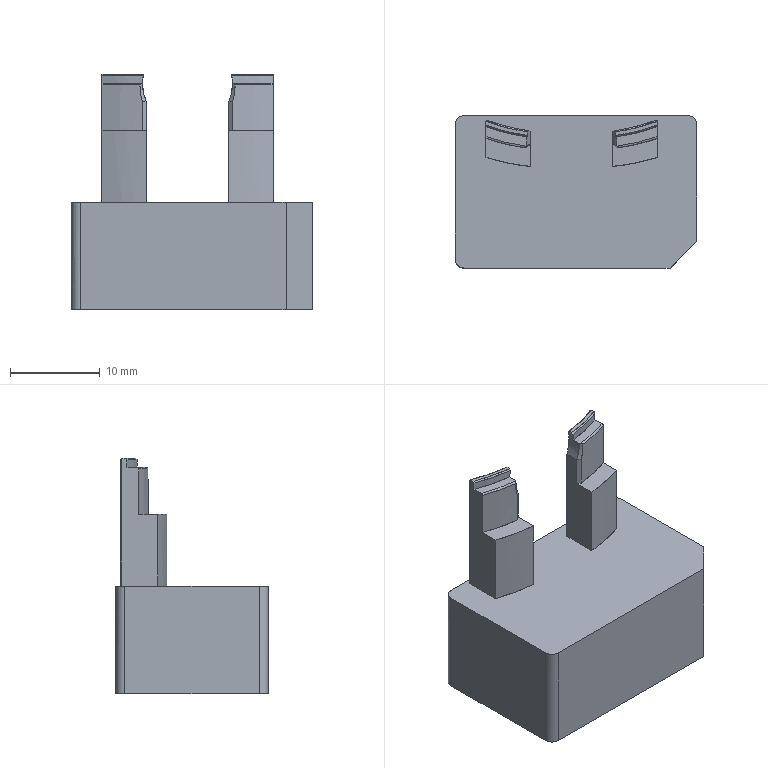NC program | PowerMill | posted by the shop | part box 27 x 17 x 26.255 mm
Lines 6760 to 8398 of 169183:
( TOOL ID   D3C_1_1 )
( TOOL DIA. 3. TIP RAD 0 LENGTH 69.44 )
( Z = -14.38 )
T15 M6
T3
G91 G28 Z0
G0 G90 G54
M08
S18000 M3
X0 Y0 M8
G43 Z9.805 H15
X-7.381 Y9.693
Z.857
G1 Z-.343 F3000
X-7.393 Y9.677 F5000
G3 X-7.362 Y9.434 I.137 J-.106
G1 X-6.118 Y8.476
X-5.066 Y8.271
X-4.643 Y8.086
X-4.32 Y7.809
X-4.221 Y7.684
X-4.059 Y7.387
X-3.949 Y6.965
X-3.924 Y6.543
X-3.932 Y6.121
X-4.017 Y5.699
X-4.221 Y5.28
X-4.675 Y4.855
X-5.066 Y4.689
X-5.488 Y4.639
X-6.754 Y4.824
X-8.021 Y5.089
X-9.287 Y5.43
X-10.553 Y5.853
X-10.975 Y6.085
X-11.398 Y6.604
X-11.518 Y6.965
X-11.552 Y7.387
Y7.809
X-11.511 Y8.232
X-11.347 Y8.654
X-11.004 Y9.076
X-10.553 Y9.353
X-10.131 Y9.46
X-9.709 Y9.452
X-8.556 Y9.076
X-7.176 Y8.683
X-7.17 Y8.682
X-6.118 Y8.476
X-7.382 Y9.701 Z-.481
X-7.394 Y9.686
G3 X-7.363 Y9.443 I.137 J-.106
G1 X-6.117 Y8.478
X-5.066 Y8.271
X-4.643 Y8.086
X-4.32 Y7.809
X-4.221 Y7.684
X-4.059 Y7.387
X-3.949 Y6.965
X-3.924 Y6.543
X-3.932 Y6.121
X-4.017 Y5.699
X-4.221 Y5.277
X-4.424 Y5.042
X-4.671 Y4.855
X-5.066 Y4.686
X-5.488 Y4.636
X-6.332 Y4.749
X-7.024 Y4.879
X-7.712 Y5.025
X-8.021 Y5.086
X-9.287 Y5.427
X-10.553 Y5.85
X-10.975 Y6.082
X-11.398 Y6.601
X-11.521 Y6.965
X-11.552 Y7.387
Y7.809
X-11.511 Y8.232
X-11.347 Y8.654
X-11.004 Y9.076
X-10.553 Y9.353
X-10.131 Y9.46
X-9.709 Y9.452
X-9.287 Y9.334
X-8.545 Y9.076
X-7.176 Y8.688
X-6.117 Y8.478
X-7.37 Y9.699 Z-.619
X-7.382 Y9.684
G3 X-7.351 Y9.44 I.137 J-.106
G1 X-6.117 Y8.481
X-5.066 Y8.271
X-4.643 Y8.086
X-4.32 Y7.809
X-4.221 Y7.684
X-4.059 Y7.387
X-3.949 Y6.965
X-3.924 Y6.543
X-3.932 Y6.121
X-4.017 Y5.699
X-4.221 Y5.277
X-4.424 Y5.042
X-4.671 Y4.855
X-5.066 Y4.686
X-5.488 Y4.636
X-6.332 Y4.749
X-6.585 Y4.799
X-6.589 Y4.8
X-6.754 Y4.824
X-7.704 Y5.023
X-8.021 Y5.086
X-9.287 Y5.427
X-10.553 Y5.85
X-10.975 Y6.082
X-11.36 Y6.543
X-11.374 Y6.575
X-11.398 Y6.601
X-11.504 Y6.917
X-11.524 Y6.969
X-11.525 Y7.025
X-11.552 Y7.387
Y7.808
Y7.809
X-11.511 Y8.232
X-11.347 Y8.654
X-11.004 Y9.076
X-10.553 Y9.353
X-10.131 Y9.46
X-9.709 Y9.452
X-9.287 Y9.334
X-8.544 Y9.076
X-7.176 Y8.692
X-6.117 Y8.481
X-7.364 Y9.698 Z-.756
X-7.376 Y9.683
G3 X-7.346 Y9.44 I.137 J-.106
G1 X-6.117 Y8.482
X-5.066 Y8.271
X-4.643 Y8.086
X-4.32 Y7.809
X-4.221 Y7.684
X-4.059 Y7.387
X-3.949 Y6.965
X-3.924 Y6.543
X-3.932 Y6.121
X-4.017 Y5.699
X-4.221 Y5.277
X-4.424 Y5.042
X-4.671 Y4.855
X-5.066 Y4.686
X-5.488 Y4.636
X-6.332 Y4.749
X-6.586 Y4.8
X-6.59
X-6.754 Y4.824
X-7.697 Y5.022
X-8.021 Y5.086
X-9.287 Y5.427
X-10.553 Y5.85
X-10.975 Y6.082
X-11.362 Y6.543
X-11.375 Y6.575
X-11.398 Y6.602
X-11.458 Y6.785
X-11.525 Y6.965
X-11.534 Y7.177
X-11.552 Y7.387
Y7.806
Y7.809
X-11.511 Y8.232
X-11.347 Y8.654
X-11.004 Y9.076
X-10.553 Y9.353
X-10.131 Y9.46
X-9.709 Y9.452
X-9.287 Y9.334
X-8.543 Y9.076
X-7.176 Y8.695
X-6.117 Y8.482
X-7.364 Y9.698 Z-.894
X-7.375 Y9.683
G3 X-7.345 Y9.44 I.137 J-.107
G1 X-6.117 Y8.482
X-5.066 Y8.271
X-4.643 Y8.086
X-4.32 Y7.809
X-4.221 Y7.684
X-4.059 Y7.387
X-3.949 Y6.965
X-3.924 Y6.543
X-3.932 Y6.121
X-4.017 Y5.699
X-4.221 Y5.277
X-4.424 Y5.042
X-4.671 Y4.855
X-5.066 Y4.686
X-5.488 Y4.636
X-6.332 Y4.749
X-7.177 Y4.912
X-8.021 Y5.086
X-9.287 Y5.427
X-10.553 Y5.85
X-10.975 Y6.082
X-11.364 Y6.543
X-11.376 Y6.575
X-11.397 Y6.602
X-11.459 Y6.785
X-11.528 Y6.965
X-11.535 Y7.177
X-11.552 Y7.387
Y7.804
Y7.809
X-11.511 Y8.232
X-11.347 Y8.654
X-11.004 Y9.076
X-10.553 Y9.353
X-10.131 Y9.46
X-9.709 Y9.452
X-9.287 Y9.334
X-8.542 Y9.076
X-7.176 Y8.695
X-7.171 Y8.694
X-6.117 Y8.482
X-7.363 Y9.699 Z-1.032
X-7.375 Y9.684
G3 X-7.345 Y9.441 I.137 J-.107
G1 X-6.117 Y8.482
X-5.066 Y8.271
X-4.643 Y8.086
X-4.32 Y7.809
X-4.221 Y7.684
X-4.059 Y7.387
X-3.949 Y6.965
X-3.924 Y6.543
X-3.932 Y6.121
X-4.017 Y5.699
X-4.221 Y5.277
X-4.424 Y5.042
X-4.671 Y4.855
X-5.066 Y4.686
X-5.488 Y4.636
X-6.332 Y4.749
X-7.009 Y4.877
X-7.683 Y5.019
X-8.021 Y5.086
X-9.287 Y5.427
X-10.553 Y5.85
X-10.975 Y6.082
X-11.366 Y6.543
X-11.418 Y6.656
X-11.456 Y6.773
X-11.53 Y6.965
X-11.536 Y7.177
X-11.552 Y7.387
Y7.802
Y7.809
X-11.511 Y8.232
X-11.347 Y8.654
X-11.004 Y9.076
X-10.553 Y9.353
X-10.131 Y9.46
X-9.709 Y9.452
X-9.287 Y9.334
X-8.515 Y9.068
X-7.319 Y8.735
X-7.176 Y8.696
X-6.117 Y8.482
X-7.367 Y9.703 Z-1.17
X-7.378 Y9.687
G3 X-7.348 Y9.444 I.137 J-.107
G1 X-6.116 Y8.483
X-5.066 Y8.271
X-4.643 Y8.086
X-4.32 Y7.809
X-4.221 Y7.684
X-4.059 Y7.387
X-3.949 Y6.965
X-3.924 Y6.543
X-3.932 Y6.121
X-4.017 Y5.699
X-4.221 Y5.277
X-4.424 Y5.042
X-4.671 Y4.855
X-5.066 Y4.686
X-5.488 Y4.636
X-6.332 Y4.749
X-7.005 Y4.876
X-7.676 Y5.017
X-8.021 Y5.086
X-9.287 Y5.427
X-10.553 Y5.85
X-10.557 Y5.852
X-10.975 Y6.082
X-10.999 Y6.106
X-11.03 Y6.121
X-11.369 Y6.543
X-11.408 Y6.633
X-11.439 Y6.726
X-11.532 Y6.965
X-11.548 Y7.387
X-11.552 Y7.809
X-11.511 Y8.232
X-11.347 Y8.654
X-11.004 Y9.076
X-10.553 Y9.353
X-10.131 Y9.46
X-9.709 Y9.452
X-9.287 Y9.334
X-8.491 Y9.062
X-7.534 Y8.795
X-7.176 Y8.696
X-6.116 Y8.483
X-7.366 Y9.702 Z-1.32
X-7.378 Y9.687
G3 X-7.348 Y9.444 I.137 J-.107
G1 X-6.116 Y8.483
X-5.066 Y8.271
X-4.643 Y8.086
X-4.32 Y7.809
X-4.221 Y7.684
X-4.059 Y7.387
X-3.949 Y6.965
X-3.923 Y6.543
X-3.932 Y6.121
X-4.017 Y5.699
Y5.688
X-4.057 Y4.855
X-4.221 Y4.432
X-4.643 Y3.953
X-5.153 Y3.588
X-5.488 Y3.475
X-5.91 Y3.447
X-7.598 Y3.74
X-9.287 Y4.154
X-10.553 Y4.552
X-10.975 Y4.784
X-11.059 Y4.855
X-11.384 Y5.277
X-11.527 Y5.699
X-11.552 Y6.121
Y7.809
X-11.511 Y8.232
X-11.347 Y8.654
X-11.004 Y9.076
X-10.553 Y9.353
X-10.131 Y9.46
X-9.709 Y9.452
X-9.287 Y9.334
X-8.532 Y9.076
X-7.176 Y8.697
X-7.171 Y8.696
X-6.116 Y8.483
X-7.366 Y9.702 Z-1.47
X-7.378 Y9.687
G3 X-7.348 Y9.444 I.137 J-.107
G1 X-6.116 Y8.483
X-5.066 Y8.271
X-4.643 Y8.086
X-4.32 Y7.809
X-4.221 Y7.684
X-4.059 Y7.387
X-3.949 Y6.965
X-3.923 Y6.543
X-3.932 Y6.121
X-4.008 Y5.699
X-4.014 Y5.277
X-4.052 Y4.855
X-4.221 Y4.43
X-4.576 Y4.01
X-4.726 Y3.891
X-4.883 Y3.782
X-5.142 Y3.588
X-5.488 Y3.465
X-5.91 Y3.437
X-6.922 Y3.588
X-8.021 Y3.811
X-9.287 Y4.132
X-10.553 Y4.53
X-10.975 Y4.762
X-11.083 Y4.855
X-11.395 Y5.277
X-11.532 Y5.699
X-11.552 Y6.121
Y7.809
X-11.511 Y8.232
X-11.347 Y8.654
X-11.004 Y9.076
X-10.553 Y9.353
X-10.131 Y9.46
X-9.709 Y9.452
X-9.287 Y9.334
X-8.532 Y9.076
X-7.176 Y8.697
X-6.116 Y8.483
X-7.366 Y9.702 Z-1.62
X-7.378 Y9.687
G3 X-7.348 Y9.444 I.137 J-.107
G1 X-6.116 Y8.483
X-5.066 Y8.271
X-4.643 Y8.086
X-4.32 Y7.809
X-4.221 Y7.684
X-4.059 Y7.387
X-3.949 Y6.965
X-3.923 Y6.543
X-3.932 Y6.121
X-3.997 Y5.699
X-4.004 Y5.277
X-4.045 Y4.855
X-4.214 Y4.432
X-4.576 Y4.01
X-4.693 Y3.917
X-4.815 Y3.83
X-5.136 Y3.588
X-5.488 Y3.462
X-5.91 Y3.436
X-6.922 Y3.588
X-8.021 Y3.811
X-9.287 Y4.132
X-10.553 Y4.53
X-10.975 Y4.762
X-11.083 Y4.855
X-11.395 Y5.277
X-11.532 Y5.699
X-11.552 Y6.121
Y7.809
X-11.511 Y8.232
X-11.347 Y8.654
X-11.004 Y9.076
X-10.553 Y9.353
X-10.131 Y9.46
X-9.709 Y9.452
X-9.287 Y9.334
X-8.532 Y9.076
X-7.176 Y8.697
X-6.116 Y8.483
X-7.366 Y9.702 Z-1.77
X-7.378 Y9.687
G3 X-7.348 Y9.444 I.137 J-.107
G1 X-6.116 Y8.483
X-5.066 Y8.271
X-4.643 Y8.086
X-4.32 Y7.809
X-4.221 Y7.684
X-4.059 Y7.387
X-3.949 Y6.965
X-3.923 Y6.543
X-3.932 Y6.121
X-3.986 Y5.699
X-3.99 Y5.277
X-4.032 Y4.855
X-4.203 Y4.432
X-4.574 Y4.01
X-4.632 Y3.966
X-4.644 Y3.953
X-4.736 Y3.887
X-4.738 Y3.886
X-5.128 Y3.588
X-5.488 Y3.459
X-5.91 Y3.434
X-6.922 Y3.588
X-8.021 Y3.811
X-9.287 Y4.132
X-10.553 Y4.53
X-10.975 Y4.762
X-11.083 Y4.855
X-11.395 Y5.277
X-11.532 Y5.699
X-11.552 Y6.121
Y7.809
X-11.511 Y8.232
X-11.347 Y8.654
X-11.004 Y9.076
X-10.553 Y9.353
X-10.131 Y9.46
X-9.709 Y9.452
X-9.287 Y9.334
X-8.532 Y9.076
X-7.176 Y8.697
X-6.116 Y8.483
X-7.366 Y9.702 Z-1.92
X-7.378 Y9.687
G3 X-7.348 Y9.444 I.137 J-.107
G1 X-6.116 Y8.483
X-5.066 Y8.271
X-4.643 Y8.086
X-4.32 Y7.809
X-4.221 Y7.684
X-4.059 Y7.387
X-3.949 Y6.965
X-3.923 Y6.543
X-3.932 Y6.121
X-3.972 Y5.699
Y5.692
Y5.277
X-4.014 Y4.855
X-4.187 Y4.432
X-4.559 Y4.01
X-5.113 Y3.588
X-5.488 Y3.456
X-5.91 Y3.433
X-6.922 Y3.588
X-8.021 Y3.811
X-9.287 Y4.132
X-10.553 Y4.53
X-10.975 Y4.762
X-11.083 Y4.855
X-11.395 Y5.277
X-11.532 Y5.699
X-11.552 Y6.121
Y7.809
X-11.511 Y8.232
X-11.347 Y8.654
X-11.004 Y9.076
X-10.553 Y9.353
X-10.131 Y9.46
X-9.709 Y9.452
X-9.287 Y9.334
X-8.532 Y9.076
X-7.176 Y8.697
X-6.116 Y8.483
X-7.366 Y9.702 Z-2.07
X-7.378 Y9.687
G3 X-7.348 Y9.444 I.137 J-.107
G1 X-6.116 Y8.483
X-5.066 Y8.271
X-4.643 Y8.088
X-4.315 Y7.809
X-4.221 Y7.692
X-4.052 Y7.387
X-3.947 Y6.965
X-3.923 Y6.543
X-3.947 Y5.277
X-3.992 Y4.855
X-4.166 Y4.432
X-4.221 Y4.348
X-4.544 Y4.01
X-5.098 Y3.588
X-5.488 Y3.453
X-5.91 Y3.431
X-6.922 Y3.588
X-8.021 Y3.811
X-9.287 Y4.132
X-10.553 Y4.53
X-10.975 Y4.762
X-11.083 Y4.855
X-11.395 Y5.277
X-11.532 Y5.699
X-11.552 Y6.121
Y7.809
X-11.511 Y8.232
X-11.347 Y8.654
X-11.004 Y9.076
X-10.553 Y9.353
X-10.131 Y9.46
X-9.709 Y9.452
X-9.287 Y9.334
X-8.333 Y9.02
X-7.182 Y8.698
X-7.177 Y8.697
X-7.172 Y8.696
X-6.116 Y8.483
G0 Z3.857
G1 X1.786 Y5.634 F10000
G0 Z.857
G1 Z-.343 F3000
X1.912 Y5.779 F5000
X2.949 Y6.965
X3.059 Y7.387
X3.32 Y7.809
X3.799 Y8.173
X4.221 Y8.304
X5.488 Y8.537
X6.754 Y8.838
X8.021 Y9.225
X8.025 Y9.226
Y9.227
X8.443 Y9.385
X8.865 Y9.468
X9.287 Y9.435
X9.709 Y9.28
X10.004 Y9.076
X10.131 Y8.952
X10.347 Y8.654
X10.511 Y8.232
X10.552 Y7.809
Y7.387
X10.509 Y6.965
X10.36 Y6.543
X10.131 Y6.225
X9.709 Y5.919
X8.443 Y5.478
X7.176 Y5.127
X5.919 Y4.855
X4.643 Y4.65
X4.221 Y4.656
X3.799 Y4.787
X3.676 Y4.855
X3.377 Y5.091
X3.223 Y5.277
X3.017 Y5.699
X2.955 Y5.977
X2.923 Y6.543
X2.949 Y6.965
X1.786 Y5.634 Z-.481
X1.912 Y5.779
X2.949 Y6.965
X3.059 Y7.387
X3.32 Y7.809
X3.799 Y8.173
X4.221 Y8.304
X5.694 Y8.586
X6.368 Y8.747
X7.038 Y8.924
X7.367 Y9.025
X7.369 Y9.026
X8.443 Y9.387
X8.865 Y9.468
X9.287 Y9.435
X9.709 Y9.28
X10.004 Y9.076
X10.131 Y8.952
X10.347 Y8.654
X10.511 Y8.232
X10.552 Y7.809
Y7.387
X10.511 Y6.965
X10.362 Y6.543
X10.131 Y6.222
X9.709 Y5.916
X8.443 Y5.475
X7.176 Y5.124
X5.936 Y4.855
X4.643 Y4.648
X4.221 Y4.653
X3.799 Y4.785
X3.671 Y4.855
X3.377 Y5.089
X3.222 Y5.277
X3.017 Y5.699
X2.955 Y5.977
X2.923 Y6.543
X2.949 Y6.965
X1.786 Y5.634 Z-.619
X1.912 Y5.779
X2.949 Y6.965
X3.059 Y7.387
X3.32 Y7.809
X3.799 Y8.173
X3.94 Y8.232
X4.083 Y8.261
X4.221 Y8.304
X5.565 Y8.561
X5.865 Y8.624
X6.162 Y8.697
X7.057 Y8.93
X7.352 Y9.02
X7.354 Y9.021
X8.443 Y9.387
X8.865 Y9.468
X9.287 Y9.435
X9.709 Y9.28
X10.004 Y9.076
X10.131 Y8.952
X10.347 Y8.654
X10.511 Y8.232
X10.552 Y7.809
Y7.387
X10.514 Y6.965
X10.365 Y6.543
X10.131 Y6.222
X9.709 Y5.916
X8.443 Y5.475
X7.176 Y5.124
X5.936 Y4.855
X4.643 Y4.648
X4.221 Y4.653
X3.799 Y4.785
X3.671 Y4.855
X3.377 Y5.089
X3.222 Y5.277
X3.017 Y5.699
X2.955 Y5.977
X2.923 Y6.543
X2.949 Y6.965
X1.786 Y5.634 Z-.756
X1.912 Y5.779
X2.949 Y6.965
X3.059 Y7.387
X3.32 Y7.809
X3.799 Y8.173
X3.94 Y8.232
X4.083 Y8.26
X4.221 Y8.304
X5.356 Y8.521
X5.76 Y8.605
X6.162 Y8.697
X7.057 Y8.93
X7.337 Y9.016
X7.339
X8.443 Y9.387
X8.865 Y9.468
X9.287 Y9.435
X9.709 Y9.28
X10.004 Y9.076
X10.131 Y8.952
X10.347 Y8.654
X10.511 Y8.232
X10.552 Y7.809
Y7.387
X10.516 Y6.965
X10.367 Y6.543
X10.131 Y6.222
X10.018 Y6.121
X9.709 Y5.916
X8.443 Y5.475
X7.176 Y5.124
X5.936 Y4.855
X4.643 Y4.647
X4.221 Y4.653
X3.799 Y4.785
X3.671 Y4.855
X3.377 Y5.089
X3.222 Y5.277
X3.017 Y5.699
X2.955 Y5.977
X2.923 Y6.543
X2.949 Y6.965
X1.786 Y5.634 Z-.894
X1.912 Y5.779
X2.949 Y6.965
X3.059 Y7.387
X3.32 Y7.809
X3.799 Y8.173
X3.94 Y8.232
X4.082 Y8.261
X4.221 Y8.304
X5.194 Y8.491
X6.162 Y8.697
X7.057 Y8.93
X7.321 Y9.011
X7.323
X8.443 Y9.387
X8.865 Y9.468
X9.287 Y9.435
X9.709 Y9.28
X10.004 Y9.076
X10.131 Y8.952
X10.347 Y8.654
X10.511 Y8.232
X10.552 Y7.809
Y7.387
X10.518 Y6.965
X10.369 Y6.543
X10.131 Y6.222
X10.02 Y6.121
X9.709 Y5.916
X8.443 Y5.475
X7.176 Y5.124
X5.936 Y4.855
X4.643 Y4.647
X4.221 Y4.653
X3.799 Y4.785
X3.671 Y4.855
X3.377 Y5.089
X3.222 Y5.277
X3.017 Y5.699
X2.955 Y5.977
X2.923 Y6.543
X2.949 Y6.965
X1.786 Y5.634 Z-1.032
X1.912 Y5.779
X2.949 Y6.965
X3.059 Y7.387
X3.32 Y7.809
X3.799 Y8.173
X3.94 Y8.232
X4.082 Y8.261
X4.221 Y8.303
X5.194 Y8.492
X6.162 Y8.697
X7.057 Y8.93
X7.305 Y9.006
X7.307
X8.443 Y9.387
X8.865 Y9.468
X9.287 Y9.435
X9.709 Y9.28
X10.004 Y9.076
X10.131 Y8.952
X10.347 Y8.654
X10.511 Y8.232
X10.552 Y7.809
Y7.387
X10.52 Y6.965
X10.371 Y6.543
X10.131 Y6.222
X10.022 Y6.121
X9.709 Y5.916
X8.443 Y5.475
X7.176 Y5.124
X5.936 Y4.855
X4.643 Y4.647
X4.221 Y4.653
X3.799 Y4.785
X3.671 Y4.855
X3.377 Y5.089
X3.222 Y5.277
X3.017 Y5.699
X2.955 Y5.977
X2.923 Y6.543
X2.949 Y6.965
X1.759 Y5.604 Z-1.17
X1.886 Y5.749
X2.949 Y6.965
X3.059 Y7.387
X3.32 Y7.809
X3.799 Y8.173
X3.94 Y8.232
X4.082 Y8.261
X4.221 Y8.303
X5.194 Y8.492
X6.162 Y8.697
X7.021 Y8.92
X7.073 Y8.935
X7.288 Y9.001
X7.29
X8.443 Y9.387
X8.865 Y9.468
X9.287 Y9.435
X9.709 Y9.28
X10.004 Y9.076
X10.131 Y8.952
X10.347 Y8.654
X10.511 Y8.232
X10.552 Y7.809
Y7.808
Y7.387
X10.524 Y7.02
X10.522 Y6.965
X10.374 Y6.543
X10.131 Y6.222
X10.025 Y6.121
X9.709 Y5.915
X8.443 Y5.475
X7.176 Y5.124
X5.936 Y4.855
X4.643 Y4.647
X4.221 Y4.653
X3.799 Y4.785
X3.671 Y4.855
X3.377 Y5.089
X3.222 Y5.277
X3.017 Y5.699
X2.955 Y5.977
X2.923 Y6.543
X2.949 Y6.965
X1.341 Y5.126 Z-1.32
X1.468 Y5.271
X2.949 Y6.965
X3.059 Y7.387
X3.32 Y7.809
X3.799 Y8.173
X3.94 Y8.232
X4.082 Y8.261
X4.221 Y8.303
X5.194 Y8.492
X6.163 Y8.697
X6.879 Y8.883
X7.133 Y8.953
X7.135 Y8.954
X7.226 Y8.981
X8.443 Y9.387
X8.865 Y9.468
X9.287 Y9.435
X9.709 Y9.28
X10.004 Y9.076
X10.131 Y8.952
X10.347 Y8.654
X10.511 Y8.232
X10.552 Y7.809
Y6.121
X10.528 Y5.699
X10.384 Y5.277
X10.131 Y4.924
X9.709 Y4.617
X8.865 Y4.327
X7.176 Y3.867
X5.796 Y3.588
X5.066 Y3.467
X4.643 Y3.451
X4.221 Y3.557
X3.799 Y3.82
X3.377 Y4.207
X3.222 Y4.432
X3.059 Y4.855
X3.022 Y5.277
X3.017 Y5.699
X2.955 Y5.977
X2.923 Y6.543
X2.949 Y6.965
X1.339 Y5.123 Z-1.47
X1.465 Y5.268
X2.949 Y6.965
X3.059 Y7.387
X3.32 Y7.809
X3.799 Y8.173
X3.94 Y8.232
X3.956 Y8.235
X4.093 Y8.264
X4.1 Y8.266
X4.221 Y8.303
X5.195 Y8.492
X6.165 Y8.697
X6.671 Y8.828
X7.176 Y8.967
X8.443 Y9.387
X8.865 Y9.468
X9.287 Y9.435
X9.709 Y9.28
X10.004 Y9.076
X10.131 Y8.952
X10.347 Y8.654
X10.511 Y8.232
X10.552 Y7.809
Y6.121
X10.532 Y5.699
X10.395 Y5.277
X10.131 Y4.902
X9.709 Y4.596
X8.865 Y4.305
X7.598 Y3.949
X5.922 Y3.588
X5.066 Y3.451
X4.643 Y3.443
X4.221 Y3.55
X3.799 Y3.82
X3.377 Y4.207
X3.22 Y4.432
X3.052 Y4.855
X3.015 Y5.277
X3.009 Y5.699
X2.955 Y5.977
X2.923 Y6.543
X2.949 Y6.965
X1.332 Y5.115 Z-1.62
X1.458 Y5.26
X2.949 Y6.965
X3.059 Y7.387
X3.32 Y7.809
X3.799 Y8.173
X3.94 Y8.232
X4.082 Y8.261
X4.221 Y8.303
X4.828 Y8.418
X5.432 Y8.543
X6.588 Y8.808
X6.806 Y8.864
X6.853 Y8.877
X6.856 Y8.878
X8.443 Y9.387
X8.865 Y9.468
X9.287 Y9.435
X9.709 Y9.28
X10.004 Y9.076
X10.131 Y8.952
X10.347 Y8.654
X10.511 Y8.232
X10.552 Y7.809
Y6.121
X10.532 Y5.699
X10.395 Y5.277
X10.131 Y4.902
X9.709 Y4.596
X8.865 Y4.305
X7.598 Y3.949
X5.922 Y3.588
X5.066 Y3.451
X4.643 Y3.44
X4.221 Y3.546
X3.799 Y3.82
X3.377 Y4.206
X3.214 Y4.432
X3.045 Y4.855
X3.005 Y5.277
X2.996 Y5.699
X2.932 Y6.121
X2.923 Y6.543
X2.949 Y6.965
X1.325 Y5.107 Z-1.77
X1.452 Y5.252
X2.949 Y6.965
X3.059 Y7.387
X3.32 Y7.809
X3.799 Y8.173
X3.94 Y8.232
X4.082 Y8.261
X4.221 Y8.303
X4.827 Y8.418
X5.431 Y8.543
X6.59 Y8.808
X6.806 Y8.864
X6.852 Y8.877
X8.443 Y9.387
X8.865 Y9.468
X9.287 Y9.435
X9.709 Y9.28
X10.004 Y9.076
X10.131 Y8.952
X10.347 Y8.654
X10.511 Y8.232
X10.552 Y7.809
Y6.121
X10.532 Y5.699
X10.395 Y5.277
X10.131 Y4.902
X9.709 Y4.596
X8.865 Y4.305
X7.598 Y3.949
X5.922 Y3.588
X5.066 Y3.451
X4.643 Y3.436
X4.221 Y3.542
X3.799 Y3.813
X3.377 Y4.196
X3.203 Y4.432
X3.032 Y4.855
X2.988 Y5.277
X2.986 Y5.699
X2.963 Y5.91
X2.932 Y6.121
X2.923 Y6.541
Y6.543
X2.949 Y6.965
X1.31 Y5.09 Z-1.92
X1.436 Y5.235
X2.949 Y6.965
X3.059 Y7.387
X3.32 Y7.809
X3.799 Y8.173
X3.94 Y8.232
X4.082 Y8.261
X4.221 Y8.303
X4.825 Y8.418
X5.426 Y8.542
X6.592 Y8.809
X6.594
X6.806 Y8.864
X6.85 Y8.876
X8.443 Y9.387
X8.865 Y9.468
X9.287 Y9.435
X9.709 Y9.28
X10.004 Y9.076
X10.131 Y8.952
X10.347 Y8.654
X10.511 Y8.232
X10.552 Y7.809
Y6.121
X10.532 Y5.699
X10.395 Y5.277
X10.131 Y4.902
X9.709 Y4.596
X8.865 Y4.305
X7.598 Y3.949
X5.922 Y3.588
X5.066 Y3.451
X4.643 Y3.433
X4.221 Y3.539
X4.113 Y3.588
X3.799 Y3.801
X3.377 Y4.181
X3.187 Y4.432
X3.014 Y4.855
X2.972 Y5.277
X2.955 Y5.972
X2.932 Y6.121
X2.924 Y6.54
X2.923 Y6.543
X2.949 Y6.965
X1.31 Y5.054 Z-2.07
X1.435 Y5.2
X2.947 Y6.966
X3.052 Y7.387
X3.315 Y7.809
X3.377 Y7.876
X3.799 Y8.174
X3.94 Y8.232
X4.082 Y8.261
X4.221 Y8.303
X4.823 Y8.417
X5.423 Y8.541
X6.594 Y8.809
X6.806 Y8.864
X6.849 Y8.876
X6.852 Y8.877
X8.443 Y9.387
X8.865 Y9.468
X9.287 Y9.435
X9.709 Y9.28
X10.004 Y9.076
X10.131 Y8.952
X10.347 Y8.654
X10.511 Y8.232
X10.552 Y7.809
Y6.121
X10.532 Y5.699
X10.395 Y5.277
X10.131 Y4.902
X9.709 Y4.596
X8.865 Y4.305
X7.598 Y3.949
X5.922 Y3.588
X5.066 Y3.451
X4.643 Y3.43
X4.221 Y3.531
X4.098 Y3.588
X3.799 Y3.788
X3.377 Y4.161
X3.166 Y4.432
X2.992 Y4.855
X2.955 Y5.079
X2.923 Y6.543
X2.947 Y6.965
Y6.966
X1.407 Y4.947 Z-2.22
X1.522 Y5.102
X2.917 Y6.971
X2.955 Y7.181
X3.023 Y7.387
X3.289 Y7.809
X3.377 Y7.9
X3.799 Y8.182
X3.923 Y8.232
X4.114 Y8.27
X4.221 Y8.303
X4.822 Y8.417
X5.42 Y8.541
X6.596 Y8.809
X6.806 Y8.864
X6.848 Y8.876
X6.85 Y8.877
X8.443 Y9.387
X8.865 Y9.468
X9.287 Y9.435
X9.709 Y9.28
X10.004 Y9.076
X10.131 Y8.952
X10.347 Y8.654
X10.511 Y8.232
X10.552 Y7.809
Y6.121
X10.532 Y5.699
X10.395 Y5.277
X10.131 Y4.902
X9.709 Y4.596
X8.865 Y4.305
X7.598 Y3.949
X5.922 Y3.588
X5.066 Y3.451
X4.643 Y3.426
X4.221 Y3.524
X4.078 Y3.588
X3.799 Y3.773
X3.377 Y4.138
X3.14 Y4.432
X2.964 Y4.855
X2.92 Y5.277
X2.916 Y6.965
X2.917 Y6.971
G0 Z2.826
G1 X-3.221 Y7.92 F10000
G0 Z-1.02
G1 Z-2.22 F3000
X-3.239 Y7.928 F5000
G3 X-3.471 Y7.851 I-.078 J-.155
G1 X-3.916 Y6.965
X-3.919 Y5.277
X-3.964 Y4.855
X-4.141 Y4.432
X-4.221 Y4.314
X-4.521 Y4.01
X-5.078 Y3.588
X-5.488 Y3.447
X-5.91 Y3.43
X-6.922 Y3.588
X-8.021 Y3.811
X-9.287 Y4.132
X-10.553 Y4.53
X-10.975 Y4.762
X-11.083 Y4.855
X-11.395 Y5.277
X-11.532 Y5.699
X-11.552 Y6.121
Y7.809
X-11.511 Y8.232
X-11.347 Y8.654
X-11.004 Y9.076
X-10.553 Y9.353
X-10.131 Y9.46
X-9.709 Y9.452
X-9.287 Y9.334
X-8.331 Y9.02
X-7.182 Y8.698
X-7.176 Y8.697
X-7.172 Y8.696
X-5.066 Y8.273
X-4.643 Y8.102
X-4.288 Y7.809
X-4.023 Y7.387
X-3.916 Y6.965
X-3.415 Y8.256 Z-2.37
X-3.433 Y8.26
G3 X-3.639 Y8.127 I-.036 J-.169
G1 X-3.887 Y6.973
X-3.885 Y6.965
X-3.883 Y5.277
X-3.929 Y4.855
X-4.107 Y4.432
X-4.221 Y4.273
X-4.491 Y4.01
X-5.047 Y3.588
X-5.488 Y3.44
X-5.91 Y3.429
X-6.922 Y3.588
X-8.021 Y3.811
X-9.287 Y4.132
X-10.553 Y4.53
X-10.975 Y4.762
X-11.083 Y4.855
X-11.395 Y5.277
X-11.532 Y5.699
X-11.552 Y6.121
Y7.809
X-11.511 Y8.232
X-11.347 Y8.654
X-11.004 Y9.076
X-10.553 Y9.353
X-10.131 Y9.46
X-9.709 Y9.452
X-9.287 Y9.334
X-8.33 Y9.019
X-7.185 Y8.699
X-7.176 Y8.697
X-7.164 Y8.694
X-5.066 Y8.273
X-5.021 Y8.255
X-5.007 Y8.252
X-4.909 Y8.232
X-4.643 Y8.115
X-4.261 Y7.809
X-3.994 Y7.387
X-3.887 Y6.973
G0 Z2.859
G1 X1.733 Y4.666 F10000
G0 Z-1.17
G1 Z-2.37 F3000
X1.819 Y4.839 F5000
X2.885 Y6.963
Y6.965
X2.994 Y7.387
X3.26 Y7.809
X3.377 Y7.925
X3.799 Y8.19
X3.908 Y8.232
X4.136 Y8.277
X4.221 Y8.303
X4.82 Y8.417
X5.417 Y8.54
X6.598 Y8.81
X6.806 Y8.864
X6.846 Y8.875
X6.849 Y8.876
X8.443 Y9.387
X8.865 Y9.468
X9.287 Y9.435
X9.709 Y9.28
X10.004 Y9.076
X10.131 Y8.952
X10.347 Y8.654
X10.511 Y8.232
X10.552 Y7.809
Y6.121
X10.532 Y5.699
X10.395 Y5.277
X10.131 Y4.902
X9.709 Y4.596
X8.865 Y4.305
X7.598 Y3.949
X5.922 Y3.588
X5.066 Y3.451
X4.643 Y3.423
X4.221 Y3.511
X4.047 Y3.588
X3.799 Y3.749
X3.377 Y4.109
X3.107 Y4.432
X2.955 Y4.766
X2.883 Y5.277
X2.885 Y6.963
G0 Z2.897
G1 X-3.153 Y7.916 F10000
G0 Z-1.32
G1 Z-2.52 F3000
X-3.17 Y7.925 F5000
G3 X-3.403 Y7.847 I-.077 J-.155
G1 X-3.85 Y6.945
X-3.846 Y5.277
X-3.894 Y4.855
X-4.074 Y4.432
X-4.221 Y4.233
X-4.458 Y4.01
X-5.01 Y3.588
X-5.488 Y3.432
X-5.91 Y3.429
X-6.922 Y3.588
X-8.021 Y3.811
X-9.287 Y4.132
X-10.553 Y4.53
X-10.975 Y4.762
X-11.083 Y4.855
X-11.395 Y5.277
X-11.532 Y5.699
X-11.552 Y6.121
Y7.809
X-11.511 Y8.232
X-11.347 Y8.654
X-11.004 Y9.076
X-10.553 Y9.353
X-10.131 Y9.46
X-9.709 Y9.452
X-9.287 Y9.334
X-8.329 Y9.019
X-7.188 Y8.7
X-7.176 Y8.697
X-7.14 Y8.689
X-5.066 Y8.273
X-5.036 Y8.261
X-5.023 Y8.258
X-4.893 Y8.232
X-4.643 Y8.129
X-4.232 Y7.809
X-3.961 Y7.387
X-3.85 Y6.965
Y6.945
G0 Z2.897
G1 X1.7 Y4.642 F10000
G0 Z-1.32
G1 Z-2.52 F3000
X1.786 Y4.814 F5000
X2.85 Y6.928
Y6.965
X2.961 Y7.387
X3.231 Y7.809
X3.377 Y7.949
X3.799 Y8.198
X3.893 Y8.232
X4.157 Y8.283
X4.222 Y8.303
X4.819 Y8.416
X5.414 Y8.539
X6.6 Y8.81
X6.806 Y8.864
X6.845 Y8.875
X6.848 Y8.876
X8.443 Y9.387
X8.865 Y9.468
X9.287 Y9.435
X9.709 Y9.28
X10.004 Y9.076
X10.131 Y8.952
X10.347 Y8.654
X10.511 Y8.232
X10.552 Y7.809
Y6.121
X10.532 Y5.699
X10.395 Y5.277
X10.131 Y4.902
X9.709 Y4.596
X8.865 Y4.305
X7.598 Y3.949
X5.922 Y3.588
X5.066 Y3.451
X4.643 Y3.418
X4.221 Y3.497
X4.011 Y3.588
X3.799 Y3.723
X3.377 Y4.08
X3.074 Y4.432
X2.955 Y4.667
X2.894 Y4.855
X2.846 Y5.277
X2.85 Y6.928
G0 Z2.939
G1 X-3.265 Y8.005 F10000
G0 Z-1.47
G1 Z-2.67 F3000
X-3.351 Y7.833 F5000
X-3.808 Y6.913
X-3.804 Y5.277
X-3.85 Y4.855
X-4.031 Y4.432
X-4.221 Y4.187
X-4.42 Y4.01
X-4.974 Y3.588
X-5.488 Y3.423
X-5.91 Y3.429
X-6.922 Y3.588
X-8.021 Y3.811
X-9.287 Y4.132
X-10.553 Y4.53
X-10.975 Y4.762
X-11.083 Y4.855
X-11.395 Y5.277
X-11.532 Y5.699
X-11.552 Y6.121
Y7.809
X-11.511 Y8.232
X-11.347 Y8.654
X-11.004 Y9.076
X-10.553 Y9.353
X-10.131 Y9.46
X-9.709 Y9.452
X-9.287 Y9.334
X-8.328 Y9.018
X-7.191 Y8.7
X-7.176 Y8.697
X-7.072 Y8.675
X-5.066 Y8.273
X-5.051 Y8.267
X-5.038 Y8.264
X-4.877 Y8.232
X-4.643 Y8.142
X-4.221 Y7.835
X-3.921 Y7.387
X-3.808 Y6.965
Y6.913
X1.661 Y4.618
X1.748 Y4.79
X2.808 Y6.901
Y6.965
X2.921 Y7.387
X3.196 Y7.809
X3.377 Y7.975
X3.799 Y8.206
X3.977 Y8.249
X4.157 Y8.283
X4.222 Y8.303
X4.817 Y8.416
X5.412 Y8.539
X6.601 Y8.811
X6.806 Y8.864
X6.844 Y8.874
X6.846 Y8.875
X8.443 Y9.387
X8.865 Y9.468
X9.287 Y9.435
X9.709 Y9.28
X10.004 Y9.076
X10.131 Y8.952
X10.347 Y8.654
X10.511 Y8.232
X10.552 Y7.809
Y6.121
X10.532 Y5.699
X10.395 Y5.277
X10.131 Y4.902
X9.709 Y4.596
X8.865 Y4.305
X7.598 Y3.949
X5.922 Y3.588
X5.066 Y3.451
X4.643 Y3.413
X4.221 Y3.483
X3.974 Y3.588
X3.799 Y3.698
X3.377 Y4.046
X3.032 Y4.432
X2.955 Y4.573
X2.851 Y4.855
X2.805 Y5.277
X2.808 Y6.901
G0 Z2.808
G1 X-3.205 Y7.998 F10000
G0 Z-1.62
G1 Z-2.82 F3000
X-3.291 Y7.826 F5000
X-3.756 Y6.894
X-3.754 Y5.277
X-3.799 Y4.865
X-3.982 Y4.432
X-4.221 Y4.141
X-4.643 Y3.783
X-4.924 Y3.588
X-5.066 Y3.521
X-5.488 Y3.414
X-5.91 Y3.429
X-6.922 Y3.588
X-8.021 Y3.811
X-9.287 Y4.132
X-10.553 Y4.53
X-10.975 Y4.762
X-11.083 Y4.855
X-11.395 Y5.277
X-11.532 Y5.699
X-11.552 Y6.121
Y7.809
X-11.511 Y8.232
X-11.347 Y8.654
X-11.004 Y9.076
X-10.553 Y9.353
X-10.131 Y9.46
X-9.709 Y9.452
X-9.707
X-9.705 Y9.451
X-9.287 Y9.334
X-8.399 Y9.042
X-8.191 Y8.98
X-7.395 Y8.757
X-6.819 Y8.625
X-5.237 Y8.307
X-5.005 Y8.261
X-4.778 Y8.194
X-4.643 Y8.156
X-4.221 Y7.879
X-4.152 Y7.809
X-3.872 Y7.387
X-3.799 Y7.182
X-3.756 Y6.965
Y6.894
X1.609 Y4.598
X1.695 Y4.77
X2.756 Y6.883
Y6.965
X2.872 Y7.387
X2.955 Y7.548
X3.152 Y7.809
X3.377 Y8.005
X3.799 Y8.214
X4.164 Y8.285
X4.222 Y8.303
X4.816 Y8.416
X5.409 Y8.538
X6.603 Y8.811
X6.806 Y8.864
X6.842 Y8.874
X6.845 Y8.875
X8.443 Y9.387
X8.865 Y9.468
X9.287 Y9.435
X9.709 Y9.28
X10.004 Y9.076
X10.131 Y8.952
X10.347 Y8.654
X10.511 Y8.232
X10.552 Y7.809
Y6.121
X10.532 Y5.699
X10.395 Y5.277
X10.131 Y4.902
X9.709 Y4.596
X8.865 Y4.305
X7.598 Y3.949
X5.922 Y3.588
X5.066 Y3.451
X4.643 Y3.408
X4.221 Y3.466
X3.925 Y3.588
X3.799 Y3.664
X3.372 Y4.01
X2.982 Y4.432
X2.801 Y4.855
X2.753 Y5.277
X2.756 Y6.883
G0 Z2.858
G1 X-3.147 Y7.991 F10000
G0 Z-1.77
G1 Z-2.97 F3000
X-3.233 Y7.819 F5000
X-3.704 Y6.873
X-3.701 Y5.277
X-3.749 Y4.855
X-3.799 Y4.698
X-3.93 Y4.432
X-4.221 Y4.094
X-4.643 Y3.743
X-4.871 Y3.588
X-5.066 Y3.499
X-5.488 Y3.406
X-5.91 Y3.429
X-6.922 Y3.588
X-8.021 Y3.811
X-9.287 Y4.132
X-10.553 Y4.53
X-10.975 Y4.762
X-11.083 Y4.855
X-11.395 Y5.277
X-11.532 Y5.699
X-11.552 Y6.121
Y7.809
X-11.511 Y8.232
X-11.347 Y8.654
X-11.004 Y9.076
X-10.553 Y9.353
X-10.131 Y9.46
X-9.709 Y9.452
X-9.287 Y9.334
X-8.395 Y9.041
X-8.393 Y9.04
X-8.191 Y8.98
X-7.396 Y8.758
X-6.818 Y8.624
X-5.237 Y8.307
X-5.066 Y8.275
X-5.051 Y8.271
X-4.844 Y8.232
X-4.643 Y8.169
X-4.221 Y7.916
X-4.108 Y7.809
X-3.823 Y7.387
X-3.704 Y6.965
Y6.873
X1.553 Y4.571
X1.64 Y4.743
X2.704 Y6.862
Y6.965
X2.823 Y7.387
X2.955 Y7.621
X3.108 Y7.809
X3.377 Y8.031
X3.799 Y8.22
X4.603 Y8.375
X5.406 Y8.537
X6.605 Y8.812
X6.806 Y8.864
X6.841 Y8.874
X6.844
X8.443 Y9.387